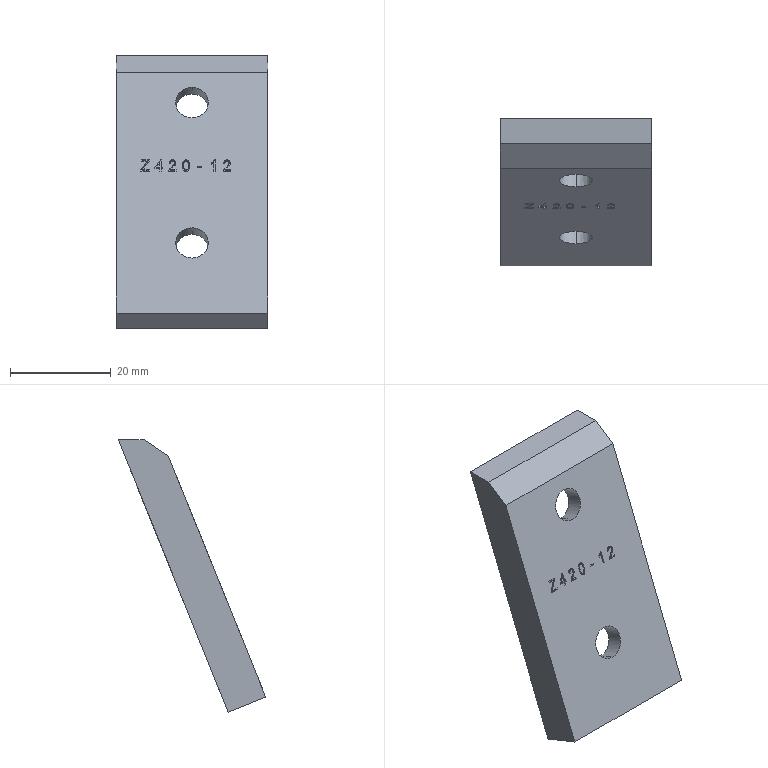Part | Creo | 1 solid | 127 faces | box 30 x 29.235 x 54 mm | volume 12292 mm3 | other 65 | plane 51 | cylinder 7 | cone 4 | commonest cylinder face diameters 6.5 x4 2.099 x2 33.097 x1